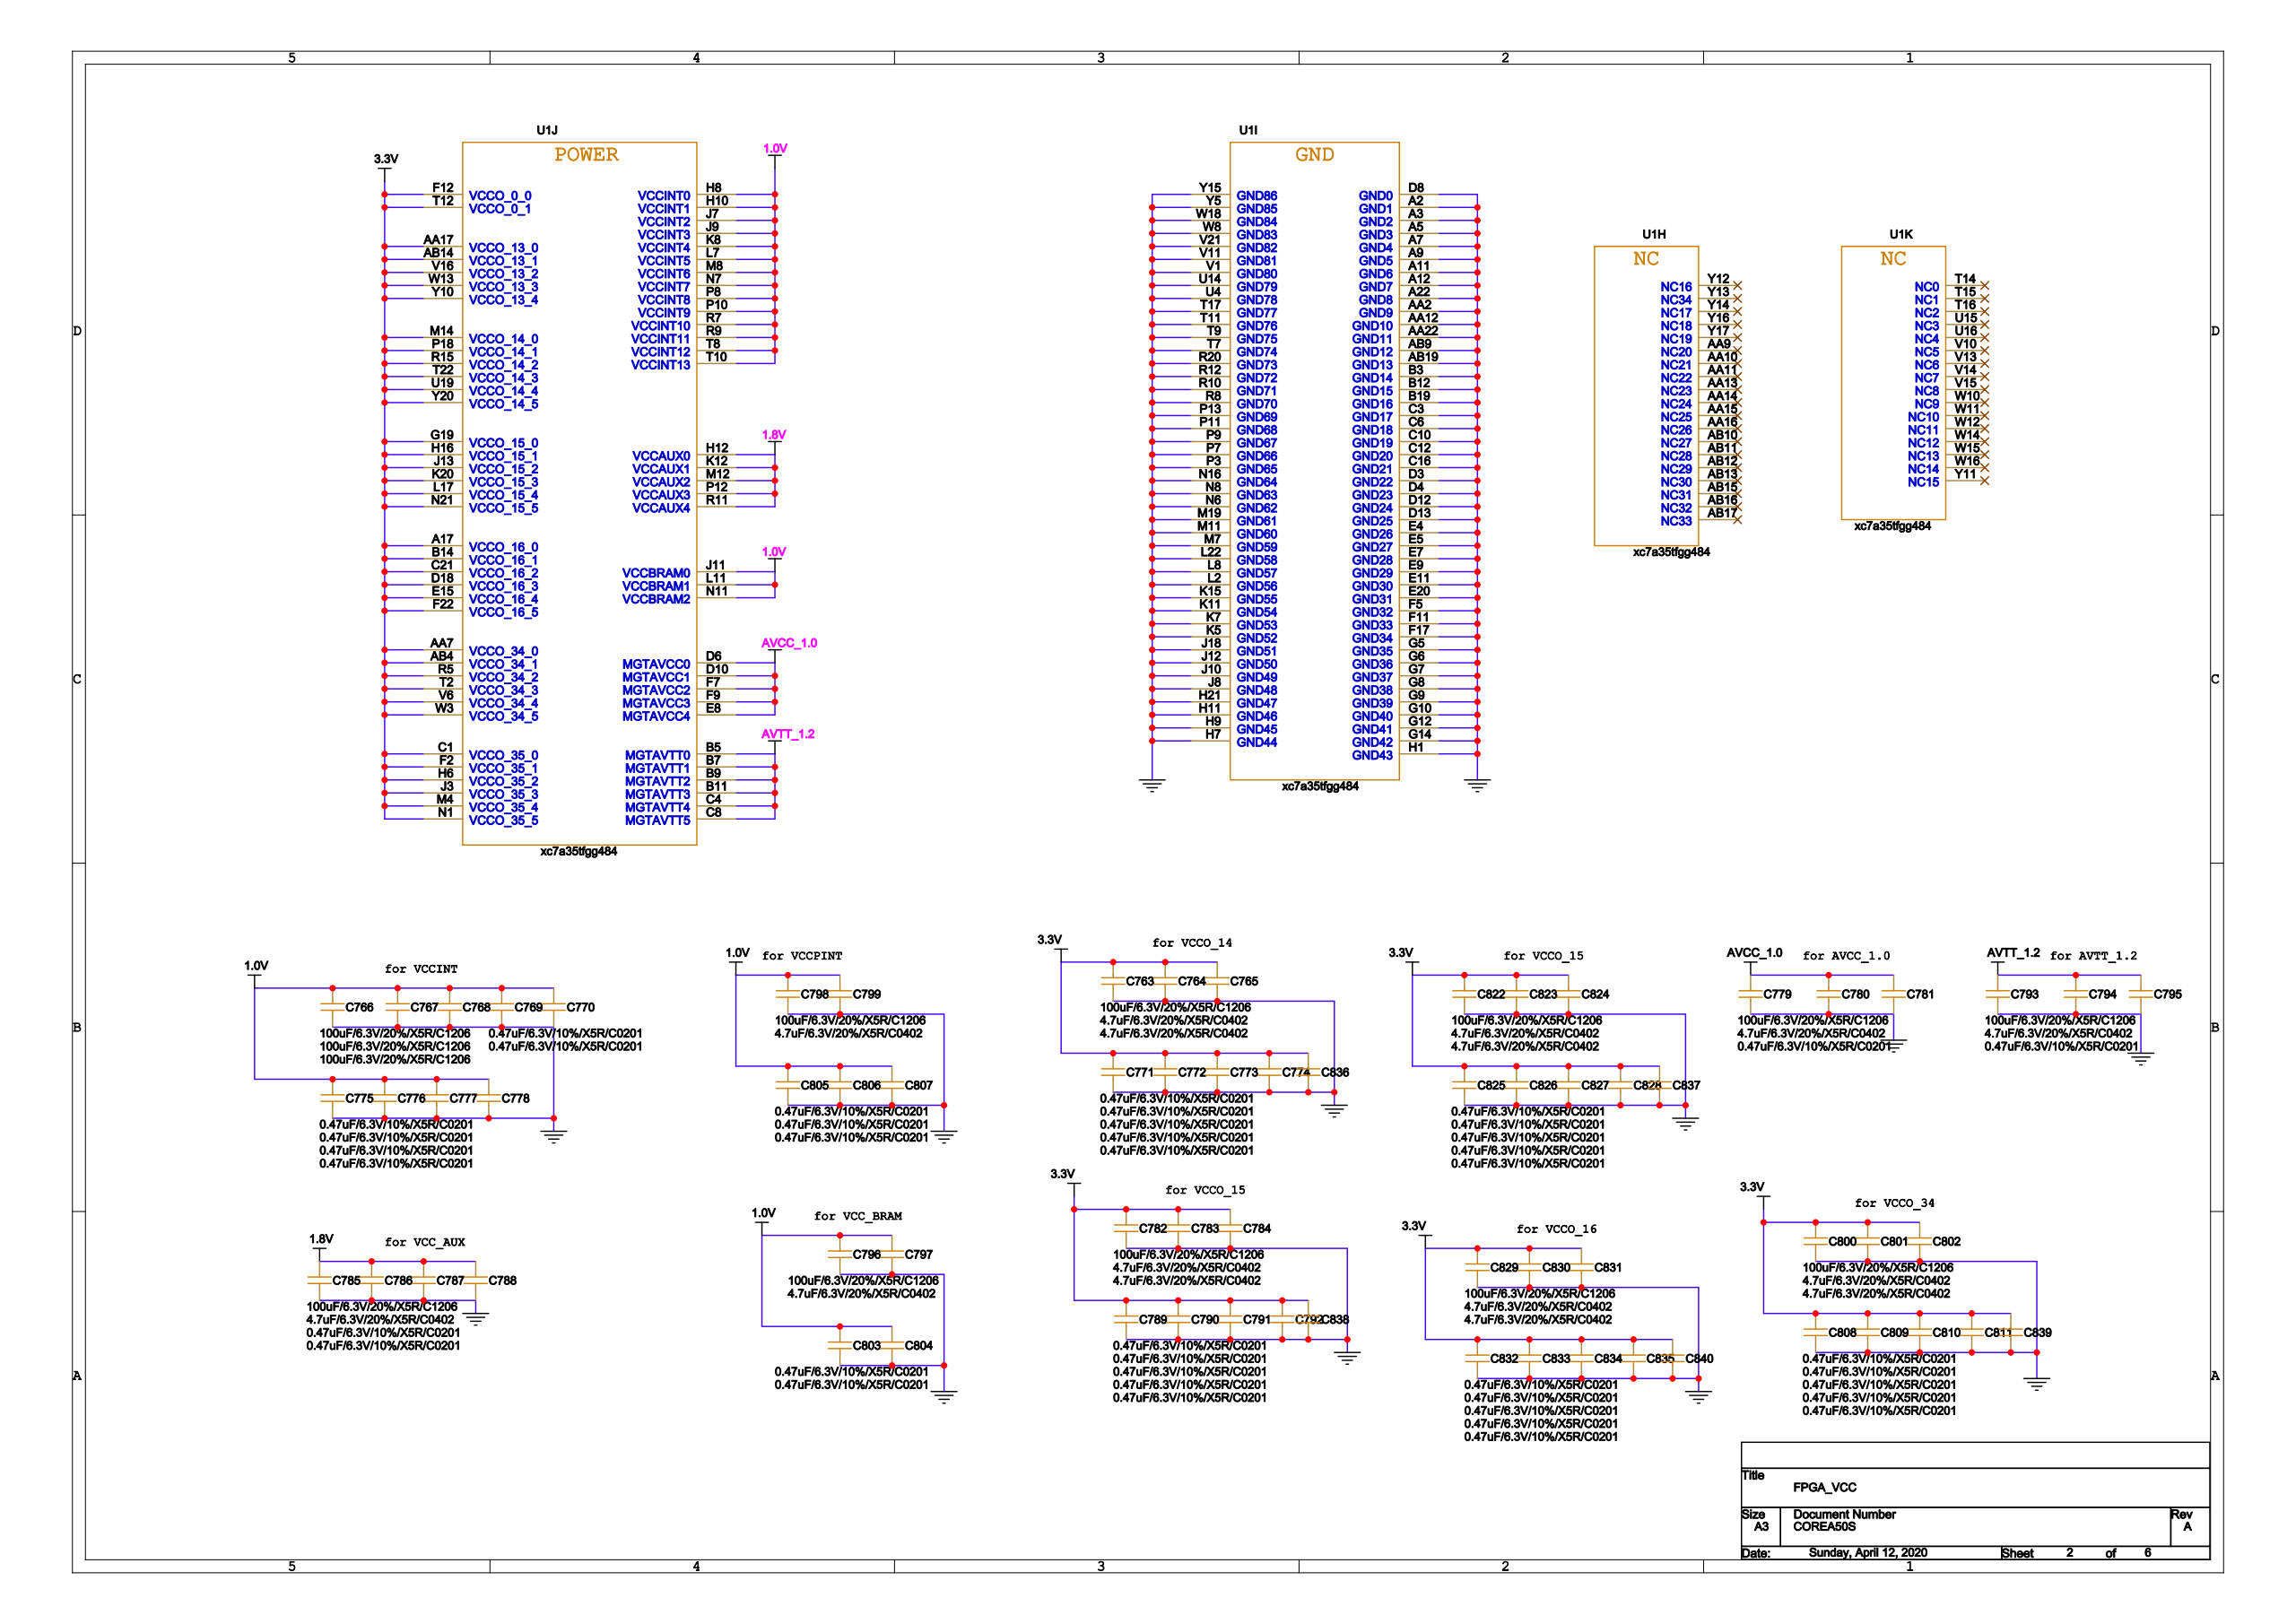Circuit board | Cadence Allegro | 202 parts | 354 nets | one sheet of the schematic
Parts on this sheet (reference | value | footprint):
C763 | 100uF/6.3V/20%/X5R/C1206 | T_1206
C764 | 4.7uF/6.3V/20%/X5R/C0402 | 0402
C765 | 4.7uF/6.3V/20%/X5R/C0402 | 0402
C766 | 100uF/6.3V/20%/X5R/C1206 | T_1206
C767 | 100uF/6.3V/20%/X5R/C1206 | T_1206
C768 | 100uF/6.3V/20%/X5R/C1206 | T_1206
C769 | 0.47uF/6.3V/10%/X5R/C0201 | 0201
C770 | 0.47uF/6.3V/10%/X5R/C0201 | 0201
C771 | 0.47uF/6.3V/10%/X5R/C0201 | 0201
C772 | 0.47uF/6.3V/10%/X5R/C0201 | 0201
C773 | 0.47uF/6.3V/10%/X5R/C0201 | 0201
C774 | 0.47uF/6.3V/10%/X5R/C0201 | 0201
C775 | 0.47uF/6.3V/10%/X5R/C0201 | 0201
C776 | 0.47uF/6.3V/10%/X5R/C0201 | 0201
C777 | 0.47uF/6.3V/10%/X5R/C0201 | 0201
C778 | 0.47uF/6.3V/10%/X5R/C0201 | 0201
C779 | 100uF/6.3V/20%/X5R/C1206 | T_1206
C780 | 4.7uF/6.3V/20%/X5R/C0402 | 0402
C781 | 0.47uF/6.3V/10%/X5R/C0201 | 0201
C782 | 100uF/6.3V/20%/X5R/C1206 | T_1206
C783 | 4.7uF/6.3V/20%/X5R/C0402 | 0402
C784 | 4.7uF/6.3V/20%/X5R/C0402 | 0402
C785 | 100uF/6.3V/20%/X5R/C1206 | T_1206
C786 | 4.7uF/6.3V/20%/X5R/C0402 | 0402
C787 | 0.47uF/6.3V/10%/X5R/C0201 | 0201
C788 | 0.47uF/6.3V/10%/X5R/C0201 | 0201
C789 | 0.47uF/6.3V/10%/X5R/C0201 | 0201
C790 | 0.47uF/6.3V/10%/X5R/C0201 | 0201
C791 | 0.47uF/6.3V/10%/X5R/C0201 | 0201
C792 | 0.47uF/6.3V/10%/X5R/C0201 | 0201
C793 | 100uF/6.3V/20%/X5R/C1206 | T_1206
C794 | 4.7uF/6.3V/20%/X5R/C0402 | 0402
C795 | 0.47uF/6.3V/10%/X5R/C0201 | 0201
C796 | 100uF/6.3V/20%/X5R/C1206 | T_1206
C797 | 4.7uF/6.3V/20%/X5R/C0402 | 0402
C798 | 100uF/6.3V/20%/X5R/C1206 | T_1206
C799 | 4.7uF/6.3V/20%/X5R/C0402 | 0402
C800 | 100uF/6.3V/20%/X5R/C1206 | T_1206
C801 | 4.7uF/6.3V/20%/X5R/C0402 | 0402
C802 | 4.7uF/6.3V/20%/X5R/C0402 | 0402
C803 | 0.47uF/6.3V/10%/X5R/C0201 | 0201
C804 | 0.47uF/6.3V/10%/X5R/C0201 | 0201
C805 | 0.47uF/6.3V/10%/X5R/C0201 | 0201
C806 | 0.47uF/6.3V/10%/X5R/C0201 | 0201
C807 | 0.47uF/6.3V/10%/X5R/C0201 | 0201
C808 | 0.47uF/6.3V/10%/X5R/C0201 | 0201
C809 | 0.47uF/6.3V/10%/X5R/C0201 | 0201
C810 | 0.47uF/6.3V/10%/X5R/C0201 | 0201
C811 | 0.47uF/6.3V/10%/X5R/C0201 | 0201
C822 | 100uF/6.3V/20%/X5R/C1206 | T_1206
C823 | 4.7uF/6.3V/20%/X5R/C0402 | 0402
C824 | 4.7uF/6.3V/20%/X5R/C0402 | 0402
C825 | 0.47uF/6.3V/10%/X5R/C0201 | 0201
C826 | 0.47uF/6.3V/10%/X5R/C0201 | 0201
C827 | 0.47uF/6.3V/10%/X5R/C0201 | 0201
C828 | 0.47uF/6.3V/10%/X5R/C0201 | 0201
C829 | 100uF/6.3V/20%/X5R/C1206 | T_1206
C830 | 4.7uF/6.3V/20%/X5R/C0402 | 0402
C831 | 4.7uF/6.3V/20%/X5R/C0402 | 0402
C832 | 0.47uF/6.3V/10%/X5R/C0201 | 0201
C833 | 0.47uF/6.3V/10%/X5R/C0201 | 0201
C834 | 0.47uF/6.3V/10%/X5R/C0201 | 0201
C835 | 0.47uF/6.3V/10%/X5R/C0201 | 0201
C836 | 0.47uF/6.3V/10%/X5R/C0201 | 0201
C837 | 0.47uF/6.3V/10%/X5R/C0201 | 0201
C838 | 0.47uF/6.3V/10%/X5R/C0201 | 0201
C839 | 0.47uF/6.3V/10%/X5R/C0201 | 0201
C840 | 0.47uF/6.3V/10%/X5R/C0201 | 0201
U1 | xc7a35tfgg484 | FGG484_23X23
Nets of these parts (net: part-pin ...):
GND: C763-2 C764-2 C765-2 C766-2 C767-2 C768-2 C769-2 C770-2 C771-2 C772-2 C773-2 C774-2 C775-2 C776-2 C777-2 C778-2 C779-2 C780-2 C781-2 C782-2 C783-2 C784-2 C785-2 C786-2 C787-2 C788-2 C789-2 C790-2 C791-2 C792-2 C793-2 C794-2 C795-2 C796-2 C797-2 C798-2 C799-2 C800-2 C801-2 C802-2 C803-2 C804-2 C805-2 C806-2 C807-2 C808-2 C809-2 C810-2 C811-2 C822-2 C823-2 C824-2 C825-2 C826-2 C827-2 C828-2 C829-2 C830-2 C831-2 C832-2 C833-2 C834-2 C835-2 C836-2 C837-2 C838-2 C839-2 C840-2 U1-A2 U1-A3 U1-A5 U1-A7 U1-A9 U1-A11 U1-A12 U1-A22 U1-AA2 U1-AA12 U1-AA22 U1-AB9 U1-AB19 U1-B3 U1-B12 U1-B19 U1-C3 U1-C6 U1-C10 U1-C12 U1-C16 U1-D3 U1-D4 U1-D8 U1-D12 U1-D13 U1-E4 U1-E5 U1-E7 U1-E9 U1-E11 U1-E20 U1-F5 U1-F11 U1-F17 U1-G5 U1-G6 U1-G7 U1-G8 U1-G9 U1-G10 U1-G12 U1-G14 U1-H1 U1-H7 U1-H9 U1-H11 U1-H21 U1-J8 U1-J10 U1-J12 U1-J18 U1-K5 U1-K7 U1-K11 U1-K15 U1-L2 U1-L8 U1-L22 U1-M7 U1-M11 U1-M19 U1-N6 U1-N8 U1-N16 U1-P3 U1-P7 U1-P9 U1-P11 U1-P13 U1-R8 U1-R10 U1-R12 U1-R20 U1-T7 U1-T9 U1-T11 U1-T17 U1-U4 U1-U14 U1-V1 U1-V11 U1-V21 U1-W8 U1-W18 U1-Y5 U1-Y15
3.3V: C763-1 C764-1 C765-1 C771-1 C772-1 C773-1 C774-1 C782-1 C783-1 C784-1 C789-1 C790-1 C791-1 C792-1 C800-1 C801-1 C802-1 C808-1 C809-1 C810-1 C811-1 C822-1 C823-1 C824-1 C825-1 C826-1 C827-1 C828-1 C829-1 C830-1 C831-1 C832-1 C833-1 C834-1 C835-1 C836-1 C837-1 C838-1 C839-1 C840-1 U1-A17 U1-AA7 U1-AA17 U1-AB4 U1-AB14 U1-B14 U1-C1 U1-C21 U1-D18 U1-E15 U1-F2 U1-F12 U1-F22 U1-G19 U1-H6 U1-H16 U1-J3 U1-J13 U1-K20 U1-L17 U1-M4 U1-M14 U1-N1 U1-N21 U1-P18 U1-R5 U1-R15 U1-T2 U1-T12 U1-T22 U1-U19 U1-V6 U1-V16 U1-W3 U1-W13 U1-Y10 U1-Y20
1.8V: C785-1 C786-1 C787-1 C788-1 U1-H12 U1-K12 U1-M12 U1-P12 U1-R11
AVCC_1.0: C779-1 C780-1 C781-1 U1-D6 U1-D10 U1-E8 U1-F7 U1-F9
AVTT_1.2: C793-1 C794-1 C795-1 U1-B5 U1-B7 U1-B9 U1-B11 U1-C4 U1-C8
1.0V: C766-1 C767-1 C768-1 C769-1 C770-1 C775-1 C776-1 C777-1 C778-1 C796-1 C797-1 C798-1 C799-1 C803-1 C804-1 C805-1 C806-1 C807-1 U1-H8 U1-H10 U1-J7 U1-J9 U1-J11 U1-K8 U1-L7 U1-L11 U1-M8 U1-N7 U1-N11 U1-P8 U1-P10 U1-R7 U1-R9 U1-T8 U1-T10